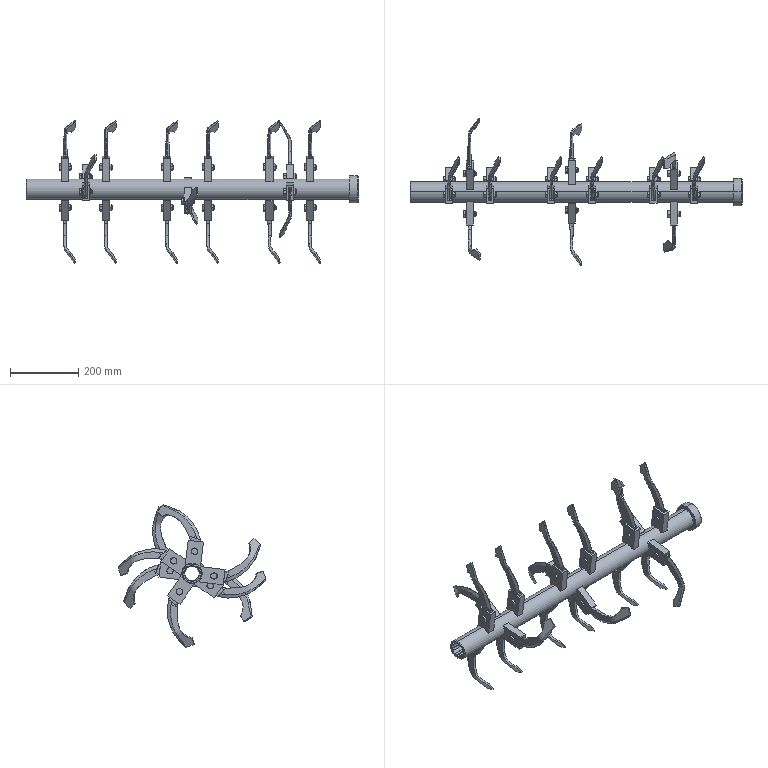Part | SolidWorks | features ReferencePattern 52, CompositeCurve 10, LocalLPattern 4, LocalCirPattern 2, AEMSimFeature 1 | 91 solids | 2189 faces | box 975 x 434.394 x 418.8 mm | volume 2976475 mm3 | plane 981 | cone 561 | spline 360 | cylinder 249 | torus 38 | commonest cylinder face diameters 12 x72 12.5 x36 13 x36 18 x36 60 x20 243.979 x18